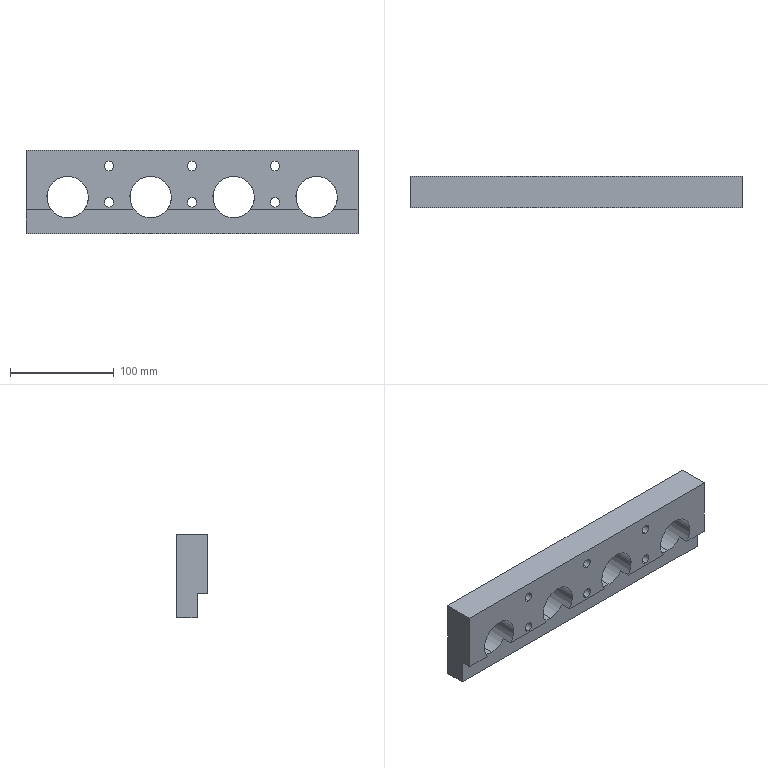Part | SolidWorks | features BaseBody 1 | 1 solid | 70 faces | box 320 x 30 x 80 mm | volume 527175 mm3 | cylinder 42 | plane 18 | cone 10 | commonest cylinder face diameters 9 x12 15 x12 8.5 x10 40 x8